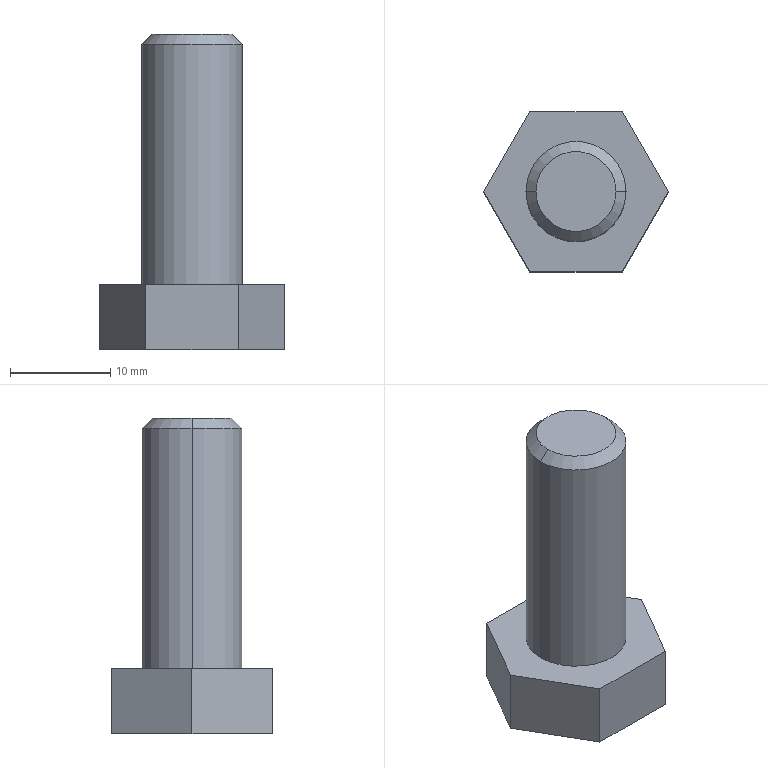Part | STEP file | Bulong M10_2.5F | 1 solid | 13 faces | box 18.475 x 16 x 31.5 mm | volume 3390 mm3 | plane 9 | cone 2 | cylinder 2 | commonest cylinder face diameters 10 x2
STEP:
#1=CARTESIAN_POINT('',(0.,0.,0.));
#2=DIRECTION('',(0.,0.,1.));
#3=DIRECTION('',(1.,0.,0.));
#4=AXIS2_PLACEMENT_3D('',#1,#2,#3);
#5=CARTESIAN_POINT('',(4.,0.,25.));
#6=VERTEX_POINT('',#5);
#7=CARTESIAN_POINT('',(-4.,0.,25.));
#8=VERTEX_POINT('',#7);
#9=CARTESIAN_POINT('',(0.,0.,25.));
#10=DIRECTION('',(0.,0.,1.));
#11=DIRECTION('',(1.,0.,0.));
#12=AXIS2_PLACEMENT_3D('',#9,#10,#11);
#13=CIRCLE('',#12,4.);
#14=CARTESIAN_POINT('',(0.,0.,25.));
#15=DIRECTION('',(0.,0.,-1.));
#16=DIRECTION('',(-1.,0.,0.));
#17=AXIS2_PLACEMENT_3D('',#14,#15,#16);
#18=CONICAL_SURFACE('',#17,4.,0.7854);
#19=CARTESIAN_POINT('',(3.142,0.));
#20=DIRECTION('',(-1.,0.));
#21=VECTOR('',#20,1.);
#22=LINE('',#19,#21);
#23=(GEOMETRIC_REPRESENTATION_CONTEXT(2)PARAMETRIC_REPRESENTATION_CONTEXT()REPRESENTATION_CONTEXT('',''));
#24=DEFINITIONAL_REPRESENTATION('',(#22),#23);
#25=PCURVE('',#18,#24);
#26=CARTESIAN_POINT('',(0.,0.,25.));
#27=DIRECTION('',(0.,0.,1.));
#28=DIRECTION('',(1.,0.,0.));
#29=AXIS2_PLACEMENT_3D('',#26,#27,#28);
#30=PLANE('',#29);
#31=CARTESIAN_POINT('',(0.,0.));
#32=DIRECTION('',(1.,0.));
#33=AXIS2_PLACEMENT_2D('',#31,#32);
#34=CIRCLE('',#33,4.);
#35=(GEOMETRIC_REPRESENTATION_CONTEXT(2)PARAMETRIC_REPRESENTATION_CONTEXT()REPRESENTATION_CONTEXT('',''));
#36=DEFINITIONAL_REPRESENTATION('',(#34),#35);
#37=PCURVE('',#30,#36);
#38=SURFACE_CURVE('',#13,(#25,#37),.PCURVE_S1.);
#39=EDGE_CURVE('',#6,#8,#38,.T.);
#40=ORIENTED_EDGE('',*,*,#39,.F.);
#41=CARTESIAN_POINT('',(5.,0.,24.));
#42=VERTEX_POINT('',#41);
#43=CARTESIAN_POINT('',(4.,0.,25.));
#44=DIRECTION('',(0.7071,0.,-0.7071));
#45=VECTOR('',#44,1.);
#46=LINE('',#43,#45);
#47=CARTESIAN_POINT('',(3.142,0.));
#48=DIRECTION('',(0.,1.));
#49=VECTOR('',#48,1.);
#50=LINE('',#47,#49);
#51=(GEOMETRIC_REPRESENTATION_CONTEXT(2)PARAMETRIC_REPRESENTATION_CONTEXT()REPRESENTATION_CONTEXT('',''));
#52=DEFINITIONAL_REPRESENTATION('',(#50),#51);
#53=PCURVE('',#18,#52);
#54=CARTESIAN_POINT('',(0.,0.,25.));
#55=DIRECTION('',(0.,0.,-1.));
#56=DIRECTION('',(-1.,0.,0.));
#57=AXIS2_PLACEMENT_3D('',#54,#55,#56);
#58=CONICAL_SURFACE('',#57,4.,0.7854);
#59=CARTESIAN_POINT('',(3.142,0.));
#60=DIRECTION('',(0.,1.));
#61=VECTOR('',#60,1.);
#62=LINE('',#59,#61);
#63=(GEOMETRIC_REPRESENTATION_CONTEXT(2)PARAMETRIC_REPRESENTATION_CONTEXT()REPRESENTATION_CONTEXT('',''));
#64=DEFINITIONAL_REPRESENTATION('',(#62),#63);
#65=PCURVE('',#58,#64);
#66=SURFACE_CURVE('',#46,(#53,#65),.PCURVE_S1.);
#67=EDGE_CURVE('',#6,#42,#66,.T.);
#68=ORIENTED_EDGE('',*,*,#67,.T.);
#69=CARTESIAN_POINT('',(-5.,0.,24.));
#70=VERTEX_POINT('',#69);
#71=CARTESIAN_POINT('',(0.,0.,24.));
#72=DIRECTION('',(0.,0.,-1.));
#73=DIRECTION('',(1.,0.,0.));
#74=AXIS2_PLACEMENT_3D('',#71,#72,#73);
#75=CIRCLE('',#74,5.);
#76=CARTESIAN_POINT('',(-3.142,1.));
#77=DIRECTION('',(1.,0.));
#78=VECTOR('',#77,1.);
#79=LINE('',#76,#78);
#80=(GEOMETRIC_REPRESENTATION_CONTEXT(2)PARAMETRIC_REPRESENTATION_CONTEXT()REPRESENTATION_CONTEXT('',''));
#81=DEFINITIONAL_REPRESENTATION('',(#79),#80);
#82=PCURVE('',#18,#81);
#83=CARTESIAN_POINT('',(0.,0.,25.));
#84=DIRECTION('',(0.,0.,-1.));
#85=DIRECTION('',(-1.,0.,0.));
#86=AXIS2_PLACEMENT_3D('',#83,#84,#85);
#87=CYLINDRICAL_SURFACE('',#86,5.);
#88=CARTESIAN_POINT('',(-3.142,1.));
#89=DIRECTION('',(1.,0.));
#90=VECTOR('',#89,1.);
#91=LINE('',#88,#90);
#92=(GEOMETRIC_REPRESENTATION_CONTEXT(2)PARAMETRIC_REPRESENTATION_CONTEXT()REPRESENTATION_CONTEXT('',''));
#93=DEFINITIONAL_REPRESENTATION('',(#91),#92);
#94=PCURVE('',#87,#93);
#95=SURFACE_CURVE('',#75,(#82,#94),.PCURVE_S1.);
#96=EDGE_CURVE('',#70,#42,#95,.T.);
#97=ORIENTED_EDGE('',*,*,#96,.F.);
#98=CARTESIAN_POINT('',(-4.,0.,25.));
#99=DIRECTION('',(-0.7071,0.,-0.7071));
#100=VECTOR('',#99,1.);
#101=LINE('',#98,#100);
#102=CARTESIAN_POINT('',(0.,0.));
#103=DIRECTION('',(0.,1.));
#104=VECTOR('',#103,1.);
#105=LINE('',#102,#104);
#106=(GEOMETRIC_REPRESENTATION_CONTEXT(2)PARAMETRIC_REPRESENTATION_CONTEXT()REPRESENTATION_CONTEXT('',''));
#107=DEFINITIONAL_REPRESENTATION('',(#105),#106);
#108=PCURVE('',#18,#107);
#109=CARTESIAN_POINT('',(6.283,0.));
#110=DIRECTION('',(0.,1.));
#111=VECTOR('',#110,1.);
#112=LINE('',#109,#111);
#113=(GEOMETRIC_REPRESENTATION_CONTEXT(2)PARAMETRIC_REPRESENTATION_CONTEXT()REPRESENTATION_CONTEXT('',''));
#114=DEFINITIONAL_REPRESENTATION('',(#112),#113);
#115=PCURVE('',#58,#114);
#116=SURFACE_CURVE('',#101,(#108,#115),.PCURVE_S1.);
#117=EDGE_CURVE('',#8,#70,#116,.T.);
#118=ORIENTED_EDGE('',*,*,#117,.F.);
#119=EDGE_LOOP('',(#40,#68,#97,#118));
#120=FACE_BOUND('',#119,.T.);
#121=ADVANCED_FACE('',(#120),#18,.T.);
#122=ORIENTED_EDGE('',*,*,#96,.T.);
#123=CARTESIAN_POINT('',(5.,0.,0.));
#124=VERTEX_POINT('',#123);
#125=CARTESIAN_POINT('',(5.,0.,25.));
#126=DIRECTION('',(0.,0.,-1.));
#127=VECTOR('',#126,1.);
#128=LINE('',#125,#127);
#129=CARTESIAN_POINT('',(3.142,0.));
#130=DIRECTION('',(0.,1.));
#131=VECTOR('',#130,1.);
#132=LINE('',#129,#131);
#133=(GEOMETRIC_REPRESENTATION_CONTEXT(2)PARAMETRIC_REPRESENTATION_CONTEXT()REPRESENTATION_CONTEXT('',''));
#134=DEFINITIONAL_REPRESENTATION('',(#132),#133);
#135=PCURVE('',#87,#134);
#136=CARTESIAN_POINT('',(0.,0.,25.));
#137=DIRECTION('',(0.,0.,-1.));
#138=DIRECTION('',(-1.,0.,0.));
#139=AXIS2_PLACEMENT_3D('',#136,#137,#138);
#140=CYLINDRICAL_SURFACE('',#139,5.);
#141=CARTESIAN_POINT('',(3.142,0.));
#142=DIRECTION('',(0.,1.));
#143=VECTOR('',#142,1.);
#144=LINE('',#141,#143);
#145=(GEOMETRIC_REPRESENTATION_CONTEXT(2)PARAMETRIC_REPRESENTATION_CONTEXT()REPRESENTATION_CONTEXT('',''));
#146=DEFINITIONAL_REPRESENTATION('',(#144),#145);
#147=PCURVE('',#140,#146);
#148=SURFACE_CURVE('',#128,(#135,#147),.PCURVE_S1.);
#149=EDGE_CURVE('',#42,#124,#148,.T.);
#150=ORIENTED_EDGE('',*,*,#149,.T.);
#151=CARTESIAN_POINT('',(-5.,0.,0.));
#152=VERTEX_POINT('',#151);
#153=CARTESIAN_POINT('',(0.,0.,0.));
#154=DIRECTION('',(0.,0.,1.));
#155=DIRECTION('',(1.,0.,0.));
#156=AXIS2_PLACEMENT_3D('',#153,#154,#155);
#157=CIRCLE('',#156,5.);
#158=CARTESIAN_POINT('',(3.142,25.));
#159=DIRECTION('',(-1.,0.));
#160=VECTOR('',#159,1.);
#161=LINE('',#158,#160);
#162=(GEOMETRIC_REPRESENTATION_CONTEXT(2)PARAMETRIC_REPRESENTATION_CONTEXT()REPRESENTATION_CONTEXT('',''));
#163=DEFINITIONAL_REPRESENTATION('',(#161),#162);
#164=PCURVE('',#87,#163);
#165=CARTESIAN_POINT('',(0.,0.,0.));
#166=DIRECTION('',(0.,0.,1.));
#167=DIRECTION('',(1.,0.,0.));
#168=AXIS2_PLACEMENT_3D('',#165,#166,#167);
#169=PLANE('',#168);
#170=CARTESIAN_POINT('',(0.,0.));
#171=DIRECTION('',(1.,0.));
#172=AXIS2_PLACEMENT_2D('',#170,#171);
#173=CIRCLE('',#172,5.);
#174=(GEOMETRIC_REPRESENTATION_CONTEXT(2)PARAMETRIC_REPRESENTATION_CONTEXT()REPRESENTATION_CONTEXT('',''));
#175=DEFINITIONAL_REPRESENTATION('',(#173),#174);
#176=PCURVE('',#169,#175);
#177=SURFACE_CURVE('',#157,(#164,#176),.PCURVE_S1.);
#178=EDGE_CURVE('',#124,#152,#177,.T.);
#179=ORIENTED_EDGE('',*,*,#178,.T.);
#180=CARTESIAN_POINT('',(-5.,0.,25.));
#181=DIRECTION('',(0.,0.,-1.));
#182=VECTOR('',#181,1.);
#183=LINE('',#180,#182);
#184=CARTESIAN_POINT('',(0.,0.));
#185=DIRECTION('',(0.,1.));
#186=VECTOR('',#185,1.);
#187=LINE('',#184,#186);
#188=(GEOMETRIC_REPRESENTATION_CONTEXT(2)PARAMETRIC_REPRESENTATION_CONTEXT()REPRESENTATION_CONTEXT('',''));
#189=DEFINITIONAL_REPRESENTATION('',(#187),#188);
#190=PCURVE('',#87,#189);
#191=CARTESIAN_POINT('',(6.283,0.));
#192=DIRECTION('',(0.,1.));
#193=VECTOR('',#192,1.);
#194=LINE('',#191,#193);
#195=(GEOMETRIC_REPRESENTATION_CONTEXT(2)PARAMETRIC_REPRESENTATION_CONTEXT()REPRESENTATION_CONTEXT('',''));
#196=DEFINITIONAL_REPRESENTATION('',(#194),#195);
#197=PCURVE('',#140,#196);
#198=SURFACE_CURVE('',#183,(#190,#197),.PCURVE_S1.);
#199=EDGE_CURVE('',#70,#152,#198,.T.);
#200=ORIENTED_EDGE('',*,*,#199,.F.);
#201=EDGE_LOOP('',(#122,#150,#179,#200));
#202=FACE_BOUND('',#201,.T.);
#203=ADVANCED_FACE('',(#202),#87,.T.);
#204=CARTESIAN_POINT('',(4.619,-8.,0.));
#205=VERTEX_POINT('',#204);
#206=CARTESIAN_POINT('',(9.238,0.,0.));
#207=VERTEX_POINT('',#206);
#208=CARTESIAN_POINT('',(4.619,-8.,0.));
#209=DIRECTION('',(0.5,0.866,0.));
#210=VECTOR('',#209,1.);
#211=LINE('',#208,#210);
#212=CARTESIAN_POINT('',(4.619,-8.));
#213=DIRECTION('',(0.5,0.866));
#214=VECTOR('',#213,1.);
#215=LINE('',#212,#214);
#216=(GEOMETRIC_REPRESENTATION_CONTEXT(2)PARAMETRIC_REPRESENTATION_CONTEXT()REPRESENTATION_CONTEXT('',''));
#217=DEFINITIONAL_REPRESENTATION('',(#215),#216);
#218=PCURVE('',#169,#217);
#219=CARTESIAN_POINT('',(4.619,-8.,-6.5));
#220=DIRECTION('',(0.866,-0.5,0.));
#221=DIRECTION('',(0.5,0.866,0.));
#222=AXIS2_PLACEMENT_3D('',#219,#220,#221);
#223=PLANE('',#222);
#224=CARTESIAN_POINT('',(0.,6.5));
#225=DIRECTION('',(1.,0.));
#226=VECTOR('',#225,1.);
#227=LINE('',#224,#226);
#228=(GEOMETRIC_REPRESENTATION_CONTEXT(2)PARAMETRIC_REPRESENTATION_CONTEXT()REPRESENTATION_CONTEXT('',''));
#229=DEFINITIONAL_REPRESENTATION('',(#227),#228);
#230=PCURVE('',#223,#229);
#231=SURFACE_CURVE('',#211,(#218,#230),.PCURVE_S1.);
#232=EDGE_CURVE('',#205,#207,#231,.T.);
#233=ORIENTED_EDGE('',*,*,#232,.T.);
#234=CARTESIAN_POINT('',(4.619,8.,0.));
#235=VERTEX_POINT('',#234);
#236=CARTESIAN_POINT('',(9.238,0.,0.));
#237=DIRECTION('',(-0.5,0.866,0.));
#238=VECTOR('',#237,1.);
#239=LINE('',#236,#238);
#240=CARTESIAN_POINT('',(9.238,0.));
#241=DIRECTION('',(-0.5,0.866));
#242=VECTOR('',#241,1.);
#243=LINE('',#240,#242);
#244=(GEOMETRIC_REPRESENTATION_CONTEXT(2)PARAMETRIC_REPRESENTATION_CONTEXT()REPRESENTATION_CONTEXT('',''));
#245=DEFINITIONAL_REPRESENTATION('',(#243),#244);
#246=PCURVE('',#169,#245);
#247=CARTESIAN_POINT('',(9.238,0.,-6.5));
#248=DIRECTION('',(0.866,0.5,0.));
#249=DIRECTION('',(-0.5,0.866,0.));
#250=AXIS2_PLACEMENT_3D('',#247,#248,#249);
#251=PLANE('',#250);
#252=CARTESIAN_POINT('',(0.,6.5));
#253=DIRECTION('',(1.,0.));
#254=VECTOR('',#253,1.);
#255=LINE('',#252,#254);
#256=(GEOMETRIC_REPRESENTATION_CONTEXT(2)PARAMETRIC_REPRESENTATION_CONTEXT()REPRESENTATION_CONTEXT('',''));
#257=DEFINITIONAL_REPRESENTATION('',(#255),#256);
#258=PCURVE('',#251,#257);
#259=SURFACE_CURVE('',#239,(#246,#258),.PCURVE_S1.);
#260=EDGE_CURVE('',#207,#235,#259,.T.);
#261=ORIENTED_EDGE('',*,*,#260,.T.);
#262=CARTESIAN_POINT('',(-4.619,8.,0.));
#263=VERTEX_POINT('',#262);
#264=CARTESIAN_POINT('',(4.619,8.,0.));
#265=DIRECTION('',(-1.,0.,0.));
#266=VECTOR('',#265,1.);
#267=LINE('',#264,#266);
#268=CARTESIAN_POINT('',(4.619,8.));
#269=DIRECTION('',(-1.,0.));
#270=VECTOR('',#269,1.);
#271=LINE('',#268,#270);
#272=(GEOMETRIC_REPRESENTATION_CONTEXT(2)PARAMETRIC_REPRESENTATION_CONTEXT()REPRESENTATION_CONTEXT('',''));
#273=DEFINITIONAL_REPRESENTATION('',(#271),#272);
#274=PCURVE('',#169,#273);
#275=CARTESIAN_POINT('',(4.619,8.,-6.5));
#276=DIRECTION('',(0.,1.,0.));
#277=DIRECTION('',(0.,0.,1.));
#278=AXIS2_PLACEMENT_3D('',#275,#276,#277);
#279=PLANE('',#278);
#280=CARTESIAN_POINT('',(6.5,0.));
#281=DIRECTION('',(0.,-1.));
#282=VECTOR('',#281,1.);
#283=LINE('',#280,#282);
#284=(GEOMETRIC_REPRESENTATION_CONTEXT(2)PARAMETRIC_REPRESENTATION_CONTEXT()REPRESENTATION_CONTEXT('',''));
#285=DEFINITIONAL_REPRESENTATION('',(#283),#284);
#286=PCURVE('',#279,#285);
#287=SURFACE_CURVE('',#267,(#274,#286),.PCURVE_S1.);
#288=EDGE_CURVE('',#235,#263,#287,.T.);
#289=ORIENTED_EDGE('',*,*,#288,.T.);
#290=CARTESIAN_POINT('',(-9.238,0.,0.));
#291=VERTEX_POINT('',#290);
#292=CARTESIAN_POINT('',(-4.619,8.,0.));
#293=DIRECTION('',(-0.5,-0.866,0.));
#294=VECTOR('',#293,1.);
#295=LINE('',#292,#294);
#296=CARTESIAN_POINT('',(-4.619,8.));
#297=DIRECTION('',(-0.5,-0.866));
#298=VECTOR('',#297,1.);
#299=LINE('',#296,#298);
#300=(GEOMETRIC_REPRESENTATION_CONTEXT(2)PARAMETRIC_REPRESENTATION_CONTEXT()REPRESENTATION_CONTEXT('',''));
#301=DEFINITIONAL_REPRESENTATION('',(#299),#300);
#302=PCURVE('',#169,#301);
#303=CARTESIAN_POINT('',(-4.619,8.,-6.5));
#304=DIRECTION('',(-0.866,0.5,0.));
#305=DIRECTION('',(-0.5,-0.866,0.));
#306=AXIS2_PLACEMENT_3D('',#303,#304,#305);
#307=PLANE('',#306);
#308=CARTESIAN_POINT('',(0.,6.5));
#309=DIRECTION('',(1.,0.));
#310=VECTOR('',#309,1.);
#311=LINE('',#308,#310);
#312=(GEOMETRIC_REPRESENTATION_CONTEXT(2)PARAMETRIC_REPRESENTATION_CONTEXT()REPRESENTATION_CONTEXT('',''));
#313=DEFINITIONAL_REPRESENTATION('',(#311),#312);
#314=PCURVE('',#307,#313);
#315=SURFACE_CURVE('',#295,(#302,#314),.PCURVE_S1.);
#316=EDGE_CURVE('',#263,#291,#315,.T.);
#317=ORIENTED_EDGE('',*,*,#316,.T.);
#318=CARTESIAN_POINT('',(-4.619,-8.,0.));
#319=VERTEX_POINT('',#318);
#320=CARTESIAN_POINT('',(-9.238,0.,0.));
#321=DIRECTION('',(0.5,-0.866,0.));
#322=VECTOR('',#321,1.);
#323=LINE('',#320,#322);
#324=CARTESIAN_POINT('',(-9.238,0.));
#325=DIRECTION('',(0.5,-0.866));
#326=VECTOR('',#325,1.);
#327=LINE('',#324,#326);
#328=(GEOMETRIC_REPRESENTATION_CONTEXT(2)PARAMETRIC_REPRESENTATION_CONTEXT()REPRESENTATION_CONTEXT('',''));
#329=DEFINITIONAL_REPRESENTATION('',(#327),#328);
#330=PCURVE('',#169,#329);
#331=CARTESIAN_POINT('',(-9.238,0.,-6.5));
#332=DIRECTION('',(-0.866,-0.5,0.));
#333=DIRECTION('',(0.5,-0.866,0.));
#334=AXIS2_PLACEMENT_3D('',#331,#332,#333);
#335=PLANE('',#334);
#336=CARTESIAN_POINT('',(0.,6.5));
#337=DIRECTION('',(1.,0.));
#338=VECTOR('',#337,1.);
#339=LINE('',#336,#338);
#340=(GEOMETRIC_REPRESENTATION_CONTEXT(2)PARAMETRIC_REPRESENTATION_CONTEXT()REPRESENTATION_CONTEXT('',''));
#341=DEFINITIONAL_REPRESENTATION('',(#339),#340);
#342=PCURVE('',#335,#341);
#343=SURFACE_CURVE('',#323,(#330,#342),.PCURVE_S1.);
#344=EDGE_CURVE('',#291,#319,#343,.T.);
#345=ORIENTED_EDGE('',*,*,#344,.T.);
#346=CARTESIAN_POINT('',(-4.619,-8.,0.));
#347=DIRECTION('',(1.,0.,0.));
#348=VECTOR('',#347,1.);
#349=LINE('',#346,#348);
#350=CARTESIAN_POINT('',(-4.619,-8.));
#351=DIRECTION('',(1.,0.));
#352=VECTOR('',#351,1.);
#353=LINE('',#350,#352);
#354=(GEOMETRIC_REPRESENTATION_CONTEXT(2)PARAMETRIC_REPRESENTATION_CONTEXT()REPRESENTATION_CONTEXT('',''));
#355=DEFINITIONAL_REPRESENTATION('',(#353),#354);
#356=PCURVE('',#169,#355);
#357=CARTESIAN_POINT('',(-4.619,-8.,-6.5));
#358=DIRECTION('',(0.,-1.,0.));
#359=DIRECTION('',(0.,0.,-1.));
#360=AXIS2_PLACEMENT_3D('',#357,#358,#359);
#361=PLANE('',#360);
#362=CARTESIAN_POINT('',(-6.5,0.));
#363=DIRECTION('',(0.,1.));
#364=VECTOR('',#363,1.);
#365=LINE('',#362,#364);
#366=(GEOMETRIC_REPRESENTATION_CONTEXT(2)PARAMETRIC_REPRESENTATION_CONTEXT()REPRESENTATION_CONTEXT('',''));
#367=DEFINITIONAL_REPRESENTATION('',(#365),#366);
#368=PCURVE('',#361,#367);
#369=SURFACE_CURVE('',#349,(#356,#368),.PCURVE_S1.);
#370=EDGE_CURVE('',#319,#205,#369,.T.);
#371=ORIENTED_EDGE('',*,*,#370,.T.);
#372=EDGE_LOOP('',(#233,#261,#289,#317,#345,#371));
#373=FACE_BOUND('',#372,.T.);
#374=CARTESIAN_POINT('',(0.,0.,0.));
#375=DIRECTION('',(0.,0.,1.));
#376=DIRECTION('',(1.,0.,0.));
#377=AXIS2_PLACEMENT_3D('',#374,#375,#376);
#378=CIRCLE('',#377,5.);
#379=CARTESIAN_POINT('',(0.,0.));
#380=DIRECTION('',(1.,0.));
#381=AXIS2_PLACEMENT_2D('',#379,#380);
#382=CIRCLE('',#381,5.);
#383=(GEOMETRIC_REPRESENTATION_CONTEXT(2)PARAMETRIC_REPRESENTATION_CONTEXT()REPRESENTATION_CONTEXT('',''));
#384=DEFINITIONAL_REPRESENTATION('',(#382),#383);
#385=PCURVE('',#169,#384);
#386=CARTESIAN_POINT('',(9.425,25.));
#387=DIRECTION('',(-1.,0.));
#388=VECTOR('',#387,1.);
#389=LINE('',#386,#388);
#390=(GEOMETRIC_REPRESENTATION_CONTEXT(2)PARAMETRIC_REPRESENTATION_CONTEXT()REPRESENTATION_CONTEXT('',''));
#391=DEFINITIONAL_REPRESENTATION('',(#389),#390);
#392=PCURVE('',#140,#391);
#393=SURFACE_CURVE('',#378,(#385,#392),.PCURVE_S1.);
#394=EDGE_CURVE('',#152,#124,#393,.T.);
#395=ORIENTED_EDGE('',*,*,#394,.F.);
#396=ORIENTED_EDGE('',*,*,#178,.F.);
#397=EDGE_LOOP('',(#395,#396));
#398=FACE_BOUND('',#397,.T.);
#399=ADVANCED_FACE('',(#373,#398),#169,.T.);
#400=ORIENTED_EDGE('',*,*,#232,.F.);
#401=CARTESIAN_POINT('',(4.619,-8.,-6.5));
#402=VERTEX_POINT('',#401);
#403=CARTESIAN_POINT('',(4.619,-8.,-6.5));
#404=DIRECTION('',(0.,0.,1.));
#405=VECTOR('',#404,1.);
#406=LINE('',#403,#405);
#407=CARTESIAN_POINT('',(0.,0.));
#408=DIRECTION('',(0.,1.));
#409=VECTOR('',#408,1.);
#410=LINE('',#407,#409);
#411=(GEOMETRIC_REPRESENTATION_CONTEXT(2)PARAMETRIC_REPRESENTATION_CONTEXT()REPRESENTATION_CONTEXT('',''));
#412=DEFINITIONAL_REPRESENTATION('',(#410),#411);
#413=PCURVE('',#223,#412);
#414=CARTESIAN_POINT('',(0.,9.238));
#415=DIRECTION('',(-1.,0.));
#416=VECTOR('',#415,1.);
#417=LINE('',#414,#416);
#418=(GEOMETRIC_REPRESENTATION_CONTEXT(2)PARAMETRIC_REPRESENTATION_CONTEXT()REPRESENTATION_CONTEXT('',''));
#419=DEFINITIONAL_REPRESENTATION('',(#417),#418);
#420=PCURVE('',#361,#419);
#421=SURFACE_CURVE('',#406,(#413,#420),.PCURVE_S1.);
#422=EDGE_CURVE('',#402,#205,#421,.T.);
#423=ORIENTED_EDGE('',*,*,#422,.F.);
#424=CARTESIAN_POINT('',(9.238,0.,-6.5));
#425=VERTEX_POINT('',#424);
#426=CARTESIAN_POINT('',(4.619,-8.,-6.5));
#427=DIRECTION('',(0.5,0.866,0.));
#428=VECTOR('',#427,1.);
#429=LINE('',#426,#428);
#430=CARTESIAN_POINT('',(0.,0.));
#431=DIRECTION('',(1.,0.));
#432=VECTOR('',#431,1.);
#433=LINE('',#430,#432);
#434=(GEOMETRIC_REPRESENTATION_CONTEXT(2)PARAMETRIC_REPRESENTATION_CONTEXT()REPRESENTATION_CONTEXT('',''));
#435=DEFINITIONAL_REPRESENTATION('',(#433),#434);
#436=PCURVE('',#223,#435);
#437=CARTESIAN_POINT('',(0.,0.,-6.5));
#438=DIRECTION('',(0.,0.,1.));
#439=DIRECTION('',(1.,0.,0.));
#440=AXIS2_PLACEMENT_3D('',#437,#438,#439);
#441=PLANE('',#440);
#442=CARTESIAN_POINT('',(4.619,-8.));
#443=DIRECTION('',(0.5,0.866));
#444=VECTOR('',#443,1.);
#445=LINE('',#442,#444);
#446=(GEOMETRIC_REPRESENTATION_CONTEXT(2)PARAMETRIC_REPRESENTATION_CONTEXT()REPRESENTATION_CONTEXT('',''));
#447=DEFINITIONAL_REPRESENTATION('',(#445),#446);
#448=PCURVE('',#441,#447);
#449=SURFACE_CURVE('',#429,(#436,#448),.PCURVE_S1.);
#450=EDGE_CURVE('',#402,#425,#449,.T.);
#451=ORIENTED_EDGE('',*,*,#450,.T.);
#452=CARTESIAN_POINT('',(9.238,0.,-6.5));
#453=DIRECTION('',(0.,0.,1.));
#454=VECTOR('',#453,1.);
#455=LINE('',#452,#454);
#456=CARTESIAN_POINT('',(9.238,0.));
#457=DIRECTION('',(0.,1.));
#458=VECTOR('',#457,1.);
#459=LINE('',#456,#458);
#460=(GEOMETRIC_REPRESENTATION_CONTEXT(2)PARAMETRIC_REPRESENTATION_CONTEXT()REPRESENTATION_CONTEXT('',''));
#461=DEFINITIONAL_REPRESENTATION('',(#459),#460);
#462=PCURVE('',#223,#461);
#463=CARTESIAN_POINT('',(0.,0.));
#464=DIRECTION('',(0.,1.));
#465=VECTOR('',#464,1.);
#466=LINE('',#463,#465);
#467=(GEOMETRIC_REPRESENTATION_CONTEXT(2)PARAMETRIC_REPRESENTATION_CONTEXT()REPRESENTATION_CONTEXT('',''));
#468=DEFINITIONAL_REPRESENTATION('',(#466),#467);
#469=PCURVE('',#251,#468);
#470=SURFACE_CURVE('',#455,(#462,#469),.PCURVE_S1.);
#471=EDGE_CURVE('',#425,#207,#470,.T.);
#472=ORIENTED_EDGE('',*,*,#471,.T.);
#473=EDGE_LOOP('',(#400,#423,#451,#472));
#474=FACE_BOUND('',#473,.T.);
#475=ADVANCED_FACE('',(#474),#223,.T.);
#476=ORIENTED_EDGE('',*,*,#370,.F.);
#477=CARTESIAN_POINT('',(-4.619,-8.,-6.5));
#478=VERTEX_POINT('',#477);
#479=CARTESIAN_POINT('',(-4.619,-8.,-6.5));
#480=DIRECTION('',(0.,0.,1.));
#481=VECTOR('',#480,1.);
#482=LINE('',#479,#481);
#483=CARTESIAN_POINT('',(0.,0.));
#484=DIRECTION('',(-1.,0.));
#485=VECTOR('',#484,1.);
#486=LINE('',#483,#485);
#487=(GEOMETRIC_REPRESENTATION_CONTEXT(2)PARAMETRIC_REPRESENTATION_CONTEXT()REPRESENTATION_CONTEXT('',''));
#488=DEFINITIONAL_REPRESENTATION('',(#486),#487);
#489=PCURVE('',#361,#488);
#490=CARTESIAN_POINT('',(9.238,0.));
#491=DIRECTION('',(0.,1.));
#492=VECTOR('',#491,1.);
#493=LINE('',#490,#492);
#494=(GEOMETRIC_REPRESENTATION_CONTEXT(2)PARAMETRIC_REPRESENTATION_CONTEXT()REPRESENTATION_CONTEXT('',''));
#495=DEFINITIONAL_REPRESENTATION('',(#493),#494);
#496=PCURVE('',#335,#495);
#497=SURFACE_CURVE('',#482,(#489,#496),.PCURVE_S1.);
#498=EDGE_CURVE('',#478,#319,#497,.T.);
#499=ORIENTED_EDGE('',*,*,#498,.F.);
#500=CARTESIAN_POINT('',(-4.619,-8.,-6.5));
#501=DIRECTION('',(1.,0.,0.));
#502=VECTOR('',#501,1.);
#503=LINE('',#500,#502);
#504=CARTESIAN_POINT('',(0.,0.));
#505=DIRECTION('',(0.,1.));
#506=VECTOR('',#505,1.);
#507=LINE('',#504,#506);
#508=(GEOMETRIC_REPRESENTATION_CONTEXT(2)PARAMETRIC_REPRESENTATION_CONTEXT()REPRESENTATION_CONTEXT('',''));
#509=DEFINITIONAL_REPRESENTATION('',(#507),#508);
#510=PCURVE('',#361,#509);
#511=CARTESIAN_POINT('',(-4.619,-8.));
#512=DIRECTION('',(1.,0.));
#513=VECTOR('',#512,1.);
#514=LINE('',#511,#513);
#515=(GEOMETRIC_REPRESENTATION_CONTEXT(2)PARAMETRIC_REPRESENTATION_CONTEXT()REPRESENTATION_CONTEXT('',''));
#516=DEFINITIONAL_REPRESENTATION('',(#514),#515);
#517=PCURVE('',#441,#516);
#518=SURFACE_CURVE('',#503,(#510,#517),.PCURVE_S1.);
#519=EDGE_CURVE('',#478,#402,#518,.T.);
#520=ORIENTED_EDGE('',*,*,#519,.T.);
#521=ORIENTED_EDGE('',*,*,#422,.T.);
#522=EDGE_LOOP('',(#476,#499,#520,#521));
#523=FACE_BOUND('',#522,.T.);
#524=ADVANCED_FACE('',(#523),#361,.T.);
#525=ORIENTED_EDGE('',*,*,#344,.F.);
#526=CARTESIAN_POINT('',(-9.238,0.,-6.5));
#527=VERTEX_POINT('',#526);
#528=CARTESIAN_POINT('',(-9.238,0.,-6.5));
#529=DIRECTION('',(0.,0.,1.));
#530=VECTOR('',#529,1.);
#531=LINE('',#528,#530);
#532=CARTESIAN_POINT('',(0.,0.));
#533=DIRECTION('',(0.,1.));
#534=VECTOR('',#533,1.);
#535=LINE('',#532,#534);
#536=(GEOMETRIC_REPRESENTATION_CONTEXT(2)PARAMETRIC_REPRESENTATION_CONTEXT()REPRESENTATION_CONTEXT('',''));
#537=DEFINITIONAL_REPRESENTATION('',(#535),#536);
#538=PCURVE('',#335,#537);
#539=CARTESIAN_POINT('',(9.238,0.));
#540=DIRECTION('',(0.,1.));
#541=VECTOR('',#540,1.);
#542=LINE('',#539,#541);
#543=(GEOMETRIC_REPRESENTATION_CONTEXT(2)PARAMETRIC_REPRESENTATION_CONTEXT()REPRESENTATION_CONTEXT('',''));
#544=DEFINITIONAL_REPRESENTATION('',(#542),#543);
#545=PCURVE('',#307,#544);
#546=SURFACE_CURVE('',#531,(#538,#545),.PCURVE_S1.);
#547=EDGE_CURVE('',#527,#291,#546,.T.);
#548=ORIENTED_EDGE('',*,*,#547,.F.);
#549=CARTESIAN_POINT('',(-9.238,0.,-6.5));
#550=DIRECTION('',(0.5,-0.866,0.));
#551=VECTOR('',#550,1.);
#552=LINE('',#549,#551);
#553=CARTESIAN_POINT('',(0.,0.));
#554=DIRECTION('',(1.,0.));
#555=VECTOR('',#554,1.);
#556=LINE('',#553,#555);
#557=(GEOMETRIC_REPRESENTATION_CONTEXT(2)PARAMETRIC_REPRESENTATION_CONTEXT()REPRESENTATION_CONTEXT('',''));
#558=DEFINITIONAL_REPRESENTATION('',(#556),#557);
#559=PCURVE('',#335,#558);
#560=CARTESIAN_POINT('',(-9.238,0.));
#561=DIRECTION('',(0.5,-0.866));
#562=VECTOR('',#561,1.);
#563=LINE('',#560,#562);
#564=(GEOMETRIC_REPRESENTATION_CONTEXT(2)PARAMETRIC_REPRESENTATION_CONTEXT()REPRESENTATION_CONTEXT('',''));
#565=DEFINITIONAL_REPRESENTATION('',(#563),#564);
#566=PCURVE('',#441,#565);
#567=SURFACE_CURVE('',#552,(#559,#566),.PCURVE_S1.);
#568=EDGE_CURVE('',#527,#478,#567,.T.);
#569=ORIENTED_EDGE('',*,*,#568,.T.);
#570=ORIENTED_EDGE('',*,*,#498,.T.);
#571=EDGE_LOOP('',(#525,#548,#569,#570));
#572=FACE_BOUND('',#571,.T.);
#573=ADVANCED_FACE('',(#572),#335,.T.);
#574=ORIENTED_EDGE('',*,*,#316,.F.);
#575=CARTESIAN_POINT('',(-4.619,8.,-6.5));
#576=VERTEX_POINT('',#575);
#577=CARTESIAN_POINT('',(-4.619,8.,-6.5));
#578=DIRECTION('',(0.,0.,1.));
#579=VECTOR('',#578,1.);
#580=LINE('',#577,#579);
#581=CARTESIAN_POINT('',(0.,0.));
#582=DIRECTION('',(0.,1.));
#583=VECTOR('',#582,1.);
#584=LINE('',#581,#583);
#585=(GEOMETRIC_REPRESENTATION_CONTEXT(2)PARAMETRIC_REPRESENTATION_CONTEXT()REPRESENTATION_CONTEXT('',''));
#586=DEFINITIONAL_REPRESENTATION('',(#584),#585);
#587=PCURVE('',#307,#586);
#588=CARTESIAN_POINT('',(0.,-9.238));
#589=DIRECTION('',(1.,0.));
#590=VECTOR('',#589,1.);
#591=LINE('',#588,#590);
#592=(GEOMETRIC_REPRESENTATION_CONTEXT(2)PARAMETRIC_REPRESENTATION_CONTEXT()REPRESENTATION_CONTEXT('',''));
#593=DEFINITIONAL_REPRESENTATION('',(#591),#592);
#594=PCURVE('',#279,#593);
#595=SURFACE_CURVE('',#580,(#587,#594),.PCURVE_S1.);
#596=EDGE_CURVE('',#576,#263,#595,.T.);
#597=ORIENTED_EDGE('',*,*,#596,.F.);
#598=CARTESIAN_POINT('',(-4.619,8.,-6.5));
#599=DIRECTION('',(-0.5,-0.866,0.));
#600=VECTOR('',#599,1.);
#601=LINE('',#598,#600);
#602=CARTESIAN_POINT('',(0.,0.));
#603=DIRECTION('',(1.,0.));
#604=VECTOR('',#603,1.);
#605=LINE('',#602,#604);
#606=(GEOMETRIC_REPRESENTATION_CONTEXT(2)PARAMETRIC_REPRESENTATION_CONTEXT()REPRESENTATION_CONTEXT('',''));
#607=DEFINITIONAL_REPRESENTATION('',(#605),#606);
#608=PCURVE('',#307,#607);
#609=CARTESIAN_POINT('',(-4.619,8.));
#610=DIRECTION('',(-0.5,-0.866));
#611=VECTOR('',#610,1.);
#612=LINE('',#609,#611);
#613=(GEOMETRIC_REPRESENTATION_CONTEXT(2)PARAMETRIC_REPRESENTATION_CONTEXT()REPRESENTATION_CONTEXT('',''));
#614=DEFINITIONAL_REPRESENTATION('',(#612),#613);
#615=PCURVE('',#441,#614);
#616=SURFACE_CURVE('',#601,(#608,#615),.PCURVE_S1.);
#617=EDGE_CURVE('',#576,#527,#616,.T.);
#618=ORIENTED_EDGE('',*,*,#617,.T.);
#619=ORIENTED_EDGE('',*,*,#547,.T.);
#620=EDGE_LOOP('',(#574,#597,#618,#619));
#621=FACE_BOUND('',#620,.T.);
#622=ADVANCED_FACE('',(#621),#307,.T.);
#623=ORIENTED_EDGE('',*,*,#288,.F.);
#624=CARTESIAN_POINT('',(4.619,8.,-6.5));
#625=VERTEX_POINT('',#624);
#626=CARTESIAN_POINT('',(4.619,8.,-6.5));
#627=DIRECTION('',(0.,0.,1.));
#628=VECTOR('',#627,1.);
#629=LINE('',#626,#628);
#630=CARTESIAN_POINT('',(0.,0.));
#631=DIRECTION('',(1.,0.));
#632=VECTOR('',#631,1.);
#633=LINE('',#630,#632);
#634=(GEOMETRIC_REPRESENTATION_CONTEXT(2)PARAMETRIC_REPRESENTATION_CONTEXT()REPRESENTATION_CONTEXT('',''));
#635=DEFINITIONAL_REPRESENTATION('',(#633),#634);
#636=PCURVE('',#279,#635);
#637=CARTESIAN_POINT('',(9.238,0.));
#638=DIRECTION('',(0.,1.));
#639=VECTOR('',#638,1.);
#640=LINE('',#637,#639);
#641=(GEOMETRIC_REPRESENTATION_CONTEXT(2)PARAMETRIC_REPRESENTATION_CONTEXT()REPRESENTATION_CONTEXT('',''));
#642=DEFINITIONAL_REPRESENTATION('',(#640),#641);
#643=PCURVE('',#251,#642);
#644=SURFACE_CURVE('',#629,(#636,#643),.PCURVE_S1.);
#645=EDGE_CURVE('',#625,#235,#644,.T.);
#646=ORIENTED_EDGE('',*,*,#645,.F.);
#647=CARTESIAN_POINT('',(4.619,8.,-6.5));
#648=DIRECTION('',(-1.,0.,0.));
#649=VECTOR('',#648,1.);
#650=LINE('',#647,#649);
#651=CARTESIAN_POINT('',(0.,0.));
#652=DIRECTION('',(0.,-1.));
#653=VECTOR('',#652,1.);
#654=LINE('',#651,#653);
#655=(GEOMETRIC_REPRESENTATION_CONTEXT(2)PARAMETRIC_REPRESENTATION_CONTEXT()REPRESENTATION_CONTEXT('',''));
#656=DEFINITIONAL_REPRESENTATION('',(#654),#655);
#657=PCURVE('',#279,#656);
#658=CARTESIAN_POINT('',(4.619,8.));
#659=DIRECTION('',(-1.,0.));
#660=VECTOR('',#659,1.);
#661=LINE('',#658,#660);
#662=(GEOMETRIC_REPRESENTATION_CONTEXT(2)PARAMETRIC_REPRESENTATION_CONTEXT()REPRESENTATION_CONTEXT('',''));
#663=DEFINITIONAL_REPRESENTATION('',(#661),#662);
#664=PCURVE('',#441,#663);
#665=SURFACE_CURVE('',#650,(#657,#664),.PCURVE_S1.);
#666=EDGE_CURVE('',#625,#576,#665,.T.);
#667=ORIENTED_EDGE('',*,*,#666,.T.);
#668=ORIENTED_EDGE('',*,*,#596,.T.);
#669=EDGE_LOOP('',(#623,#646,#667,#668));
#670=FACE_BOUND('',#669,.T.);
#671=ADVANCED_FACE('',(#670),#279,.T.);
#672=ORIENTED_EDGE('',*,*,#260,.F.);
#673=ORIENTED_EDGE('',*,*,#471,.F.);
#674=CARTESIAN_POINT('',(9.238,0.,-6.5));
#675=DIRECTION('',(-0.5,0.866,0.));
#676=VECTOR('',#675,1.);
#677=LINE('',#674,#676);
#678=CARTESIAN_POINT('',(0.,0.));
#679=DIRECTION('',(1.,0.));
#680=VECTOR('',#679,1.);
#681=LINE('',#678,#680);
#682=(GEOMETRIC_REPRESENTATION_CONTEXT(2)PARAMETRIC_REPRESENTATION_CONTEXT()REPRESENTATION_CONTEXT('',''));
#683=DEFINITIONAL_REPRESENTATION('',(#681),#682);
#684=PCURVE('',#251,#683);
#685=CARTESIAN_POINT('',(9.238,0.));
#686=DIRECTION('',(-0.5,0.866));
#687=VECTOR('',#686,1.);
#688=LINE('',#685,#687);
#689=(GEOMETRIC_REPRESENTATION_CONTEXT(2)PARAMETRIC_REPRESENTATION_CONTEXT()REPRESENTATION_CONTEXT('',''));
#690=DEFINITIONAL_REPRESENTATION('',(#688),#689);
#691=PCURVE('',#441,#690);
#692=SURFACE_CURVE('',#677,(#684,#691),.PCURVE_S1.);
#693=EDGE_CURVE('',#425,#625,#692,.T.);
#694=ORIENTED_EDGE('',*,*,#693,.T.);
#695=ORIENTED_EDGE('',*,*,#645,.T.);
#696=EDGE_LOOP('',(#672,#673,#694,#695));
#697=FACE_BOUND('',#696,.T.);
#698=ADVANCED_FACE('',(#697),#251,.T.);
#699=ORIENTED_EDGE('',*,*,#450,.F.);
#700=ORIENTED_EDGE('',*,*,#519,.F.);
#701=ORIENTED_EDGE('',*,*,#568,.F.);
#702=ORIENTED_EDGE('',*,*,#617,.F.);
#703=ORIENTED_EDGE('',*,*,#666,.F.);
#704=ORIENTED_EDGE('',*,*,#693,.F.);
#705=EDGE_LOOP('',(#699,#700,#701,#702,#703,#704));
#706=FACE_BOUND('',#705,.T.);
#707=ADVANCED_FACE('',(#706),#441,.F.);
#708=ORIENTED_EDGE('',*,*,#149,.F.);
#709=CARTESIAN_POINT('',(0.,0.,24.));
#710=DIRECTION('',(0.,0.,-1.));
#711=DIRECTION('',(1.,0.,0.));
#712=AXIS2_PLACEMENT_3D('',#709,#710,#711);
#713=CIRCLE('',#712,5.);
#714=CARTESIAN_POINT('',(3.142,1.));
#715=DIRECTION('',(1.,0.));
#716=VECTOR('',#715,1.);
#717=LINE('',#714,#716);
#718=(GEOMETRIC_REPRESENTATION_CONTEXT(2)PARAMETRIC_REPRESENTATION_CONTEXT()REPRESENTATION_CONTEXT('',''));
#719=DEFINITIONAL_REPRESENTATION('',(#717),#718);
#720=PCURVE('',#140,#719);
#721=CARTESIAN_POINT('',(3.142,1.));
#722=DIRECTION('',(1.,0.));
#723=VECTOR('',#722,1.);
#724=LINE('',#721,#723);
#725=(GEOMETRIC_REPRESENTATION_CONTEXT(2)PARAMETRIC_REPRESENTATION_CONTEXT()REPRESENTATION_CONTEXT('',''));
#726=DEFINITIONAL_REPRESENTATION('',(#724),#725);
#727=PCURVE('',#58,#726);
#728=SURFACE_CURVE('',#713,(#720,#727),.PCURVE_S1.);
#729=EDGE_CURVE('',#42,#70,#728,.T.);
#730=ORIENTED_EDGE('',*,*,#729,.T.);
#731=ORIENTED_EDGE('',*,*,#199,.T.);
#732=ORIENTED_EDGE('',*,*,#394,.T.);
#733=EDGE_LOOP('',(#708,#730,#731,#732));
#734=FACE_BOUND('',#733,.T.);
#735=ADVANCED_FACE('',(#734),#140,.T.);
#736=CARTESIAN_POINT('',(0.,0.,25.));
#737=DIRECTION('',(0.,0.,1.));
#738=DIRECTION('',(1.,0.,0.));
#739=AXIS2_PLACEMENT_3D('',#736,#737,#738);
#740=CIRCLE('',#739,4.);
#741=CARTESIAN_POINT('',(0.,0.));
#742=DIRECTION('',(1.,0.));
#743=AXIS2_PLACEMENT_2D('',#741,#742);
#744=CIRCLE('',#743,4.);
#745=(GEOMETRIC_REPRESENTATION_CONTEXT(2)PARAMETRIC_REPRESENTATION_CONTEXT()REPRESENTATION_CONTEXT('',''));
#746=DEFINITIONAL_REPRESENTATION('',(#744),#745);
#747=PCURVE('',#30,#746);
#748=CARTESIAN_POINT('',(9.425,0.));
#749=DIRECTION('',(-1.,0.));
#750=VECTOR('',#749,1.);
#751=LINE('',#748,#750);
#752=(GEOMETRIC_REPRESENTATION_CONTEXT(2)PARAMETRIC_REPRESENTATION_CONTEXT()REPRESENTATION_CONTEXT('',''));
#753=DEFINITIONAL_REPRESENTATION('',(#751),#752);
#754=PCURVE('',#58,#753);
#755=SURFACE_CURVE('',#740,(#747,#754),.PCURVE_S1.);
#756=EDGE_CURVE('',#8,#6,#755,.T.);
#757=ORIENTED_EDGE('',*,*,#756,.T.);
#758=ORIENTED_EDGE('',*,*,#39,.T.);
#759=EDGE_LOOP('',(#757,#758));
#760=FACE_BOUND('',#759,.T.);
#761=ADVANCED_FACE('',(#760),#30,.T.);
#762=ORIENTED_EDGE('',*,*,#67,.F.);
#763=ORIENTED_EDGE('',*,*,#756,.F.);
#764=ORIENTED_EDGE('',*,*,#117,.T.);
#765=ORIENTED_EDGE('',*,*,#729,.F.);
#766=EDGE_LOOP('',(#762,#763,#764,#765));
#767=FACE_BOUND('',#766,.T.);
#768=ADVANCED_FACE('',(#767),#58,.T.);
#769=CLOSED_SHELL('',(#121,#203,#399,#475,#524,#573,#622,#671,#698,#707,#735,#761,#768));
#770=MANIFOLD_SOLID_BREP('',#769);
#771=(LENGTH_UNIT()NAMED_UNIT(*)SI_UNIT(.MILLI.,.METRE.));
#772=UNCERTAINTY_MEASURE_WITH_UNIT(LENGTH_MEASURE(0.0000001),#771,'','');
#773=(NAMED_UNIT(*)PLANE_ANGLE_UNIT()SI_UNIT($,.RADIAN.));
#774=(NAMED_UNIT(*)SI_UNIT($,.STERADIAN.)SOLID_ANGLE_UNIT());
#775=(GEOMETRIC_REPRESENTATION_CONTEXT(3)GLOBAL_UNCERTAINTY_ASSIGNED_CONTEXT((#772))GLOBAL_UNIT_ASSIGNED_CONTEXT((#771,#773,#774))REPRESENTATION_CONTEXT('',''));
#776=ADVANCED_BREP_SHAPE_REPRESENTATION('',(#4,#770),#775);